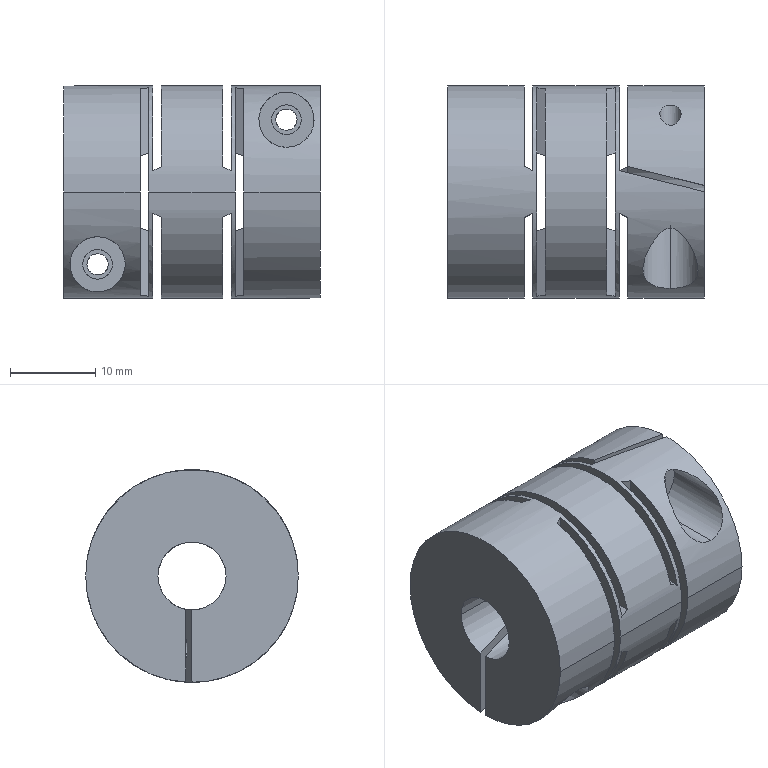Part | NX | 1 solid | 66 faces | box 30.2 x 25 x 25 mm | volume 10870 mm3 | plane 38 | cylinder 28 | commonest cylinder face diameters 3.5 x8 8 x6 2.5 x4 6.5 x4 25 x4 10.4 x2